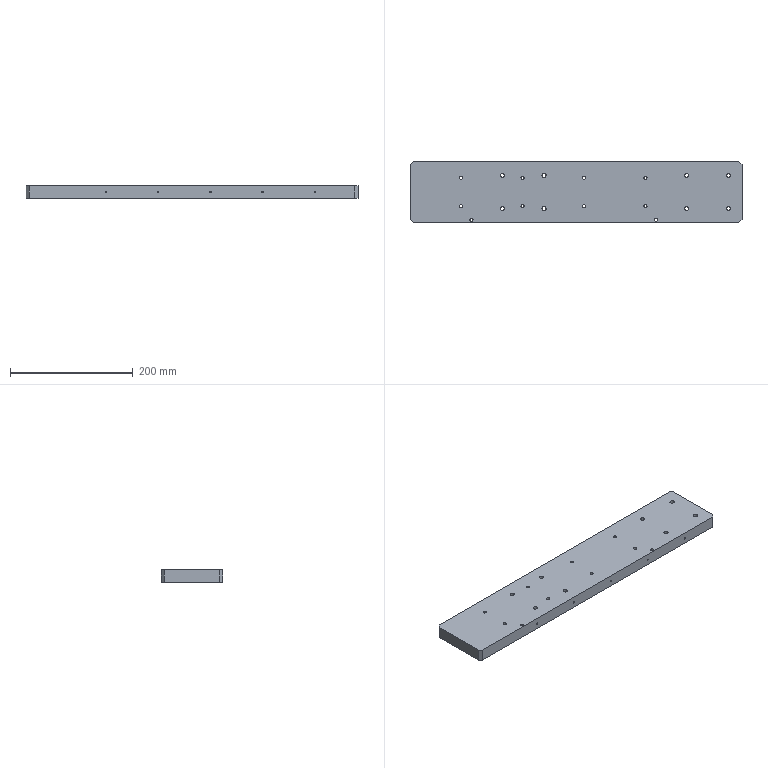Part | NX | features BREP 1 | 1 solid | 90 faces | box 540 x 100 x 20 mm | volume 1068657 mm3 | cylinder 50 | cone 30 | plane 10 | commonest cylinder face diameters 5 x20 6.8 x16 2.5 x10 4.2 x4